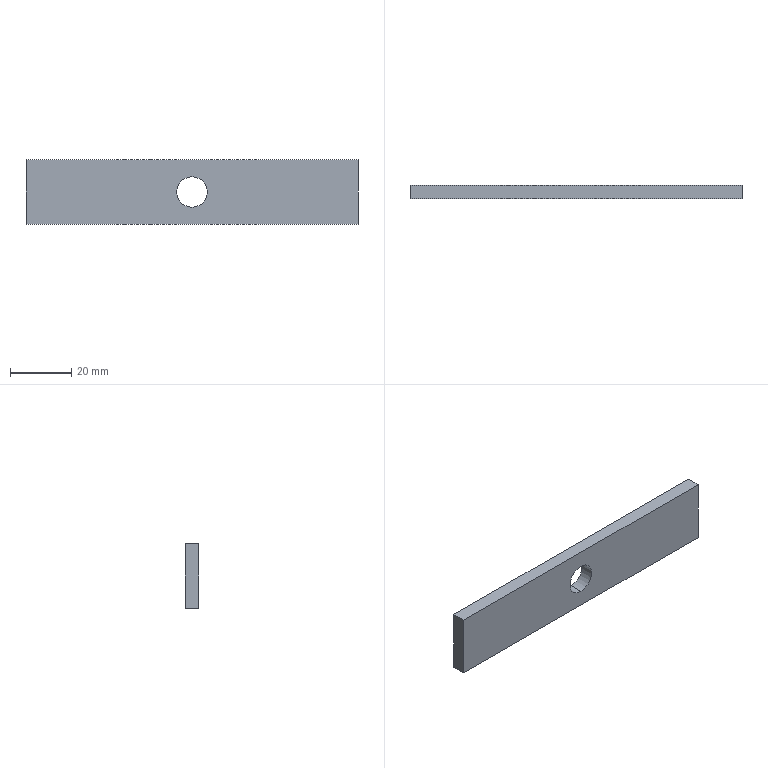Part | SolidWorks | features Extrusion 1 | 1 solid | 8 faces | box 108.732 x 4.5 x 21.168 mm | volume 10004 mm3 | plane 6 | cylinder 2 | commonest cylinder face diameters 10 x2
STEP:
#1=CARTESIAN_POINT('',(54.366,4.5,-15.584));
#2=VERTEX_POINT('',#1);
#3=CARTESIAN_POINT('',(54.366,4.5,-5.584));
#4=VERTEX_POINT('',#3);
#5=CARTESIAN_POINT('',(54.366,4.5,-10.584));
#6=DIRECTION('',(0.,1.,0.));
#7=DIRECTION('',(0.,0.,1.));
#8=AXIS2_PLACEMENT_3D('',#5,#6,#7);
#9=CIRCLE('',#8,5.);
#10=EDGE_CURVE('',#2,#4,#9,.T.);
#11=ORIENTED_EDGE('',*,*,#10,.T.);
#12=CARTESIAN_POINT('',(54.366,0.,-5.584));
#13=VERTEX_POINT('',#12);
#14=CARTESIAN_POINT('',(54.366,4.5,-5.584));
#15=DIRECTION('',(0.,-1.,0.));
#16=VECTOR('',#15,1000.);
#17=LINE('',#14,#16);
#18=EDGE_CURVE('',#4,#13,#17,.T.);
#19=ORIENTED_EDGE('',*,*,#18,.T.);
#20=CARTESIAN_POINT('',(54.366,0.,-15.584));
#21=VERTEX_POINT('',#20);
#22=CARTESIAN_POINT('',(54.366,0.,-10.584));
#23=DIRECTION('',(0.,1.,0.));
#24=DIRECTION('',(0.,0.,1.));
#25=AXIS2_PLACEMENT_3D('',#22,#23,#24);
#26=CIRCLE('',#25,5.);
#27=EDGE_CURVE('',#21,#13,#26,.T.);
#28=ORIENTED_EDGE('',*,*,#27,.F.);
#29=CARTESIAN_POINT('',(54.366,4.5,-15.584));
#30=DIRECTION('',(0.,-1.,0.));
#31=VECTOR('',#30,1000.);
#32=LINE('',#29,#31);
#33=EDGE_CURVE('',#2,#21,#32,.T.);
#34=ORIENTED_EDGE('',*,*,#33,.F.);
#35=EDGE_LOOP('',(#11,#19,#28,#34));
#36=FACE_OUTER_BOUND('',#35,.T.);
#37=CARTESIAN_POINT('',(54.366,4.5,-10.584));
#38=DIRECTION('',(0.,-1.,0.));
#39=DIRECTION('',(0.,0.,-1.));
#40=AXIS2_PLACEMENT_3D('',#37,#38,#39);
#41=CYLINDRICAL_SURFACE('',#40,5.);
#42=ADVANCED_FACE('',(#36),#41,.F.);
#43=CARTESIAN_POINT('',(0.,4.5,-21.168));
#44=VERTEX_POINT('',#43);
#45=CARTESIAN_POINT('',(0.,4.5,0.));
#46=VERTEX_POINT('',#45);
#47=CARTESIAN_POINT('',(0.,4.5,0.));
#48=DIRECTION('',(0.,0.,1.));
#49=VECTOR('',#48,1000.);
#50=LINE('',#47,#49);
#51=EDGE_CURVE('',#44,#46,#50,.T.);
#52=ORIENTED_EDGE('',*,*,#51,.T.);
#53=CARTESIAN_POINT('',(108.732,4.5,0.));
#54=VERTEX_POINT('',#53);
#55=CARTESIAN_POINT('',(0.,4.5,0.));
#56=DIRECTION('',(1.,0.,0.));
#57=VECTOR('',#56,1000.);
#58=LINE('',#55,#57);
#59=EDGE_CURVE('',#46,#54,#58,.T.);
#60=ORIENTED_EDGE('',*,*,#59,.T.);
#61=CARTESIAN_POINT('',(108.732,4.5,-21.168));
#62=VERTEX_POINT('',#61);
#63=CARTESIAN_POINT('',(108.732,4.5,0.));
#64=DIRECTION('',(0.,0.,-1.));
#65=VECTOR('',#64,1000.);
#66=LINE('',#63,#65);
#67=EDGE_CURVE('',#54,#62,#66,.T.);
#68=ORIENTED_EDGE('',*,*,#67,.T.);
#69=CARTESIAN_POINT('',(0.,4.5,-21.168));
#70=DIRECTION('',(-1.,0.,0.));
#71=VECTOR('',#70,1000.);
#72=LINE('',#69,#71);
#73=EDGE_CURVE('',#62,#44,#72,.T.);
#74=ORIENTED_EDGE('',*,*,#73,.T.);
#75=EDGE_LOOP('',(#52,#60,#68,#74));
#76=FACE_OUTER_BOUND('',#75,.T.);
#77=ORIENTED_EDGE('',*,*,#10,.F.);
#78=CARTESIAN_POINT('',(54.366,4.5,-10.584));
#79=DIRECTION('',(0.,1.,0.));
#80=DIRECTION('',(0.,0.,1.));
#81=AXIS2_PLACEMENT_3D('',#78,#79,#80);
#82=CIRCLE('',#81,5.);
#83=EDGE_CURVE('',#4,#2,#82,.T.);
#84=ORIENTED_EDGE('',*,*,#83,.F.);
#85=EDGE_LOOP('',(#77,#84));
#86=FACE_BOUND('',#85,.T.);
#87=CARTESIAN_POINT('',(0.,4.5,0.));
#88=DIRECTION('',(0.,-1.,0.));
#89=DIRECTION('',(0.,0.,-1.));
#90=AXIS2_PLACEMENT_3D('',#87,#88,#89);
#91=PLANE('',#90);
#92=ADVANCED_FACE('',(#76,#86),#91,.F.);
#93=CARTESIAN_POINT('',(0.,0.,-21.168));
#94=VERTEX_POINT('',#93);
#95=CARTESIAN_POINT('',(0.,0.,0.));
#96=VERTEX_POINT('',#95);
#97=CARTESIAN_POINT('',(0.,0.,0.));
#98=DIRECTION('',(0.,0.,1.));
#99=VECTOR('',#98,1000.);
#100=LINE('',#97,#99);
#101=EDGE_CURVE('',#94,#96,#100,.T.);
#102=ORIENTED_EDGE('',*,*,#101,.F.);
#103=CARTESIAN_POINT('',(108.732,0.,-21.168));
#104=VERTEX_POINT('',#103);
#105=CARTESIAN_POINT('',(0.,0.,-21.168));
#106=DIRECTION('',(-1.,0.,0.));
#107=VECTOR('',#106,1000.);
#108=LINE('',#105,#107);
#109=EDGE_CURVE('',#104,#94,#108,.T.);
#110=ORIENTED_EDGE('',*,*,#109,.F.);
#111=CARTESIAN_POINT('',(108.732,0.,0.));
#112=VERTEX_POINT('',#111);
#113=CARTESIAN_POINT('',(108.732,0.,0.));
#114=DIRECTION('',(0.,0.,-1.));
#115=VECTOR('',#114,1000.);
#116=LINE('',#113,#115);
#117=EDGE_CURVE('',#112,#104,#116,.T.);
#118=ORIENTED_EDGE('',*,*,#117,.F.);
#119=CARTESIAN_POINT('',(0.,0.,0.));
#120=DIRECTION('',(1.,0.,0.));
#121=VECTOR('',#120,1000.);
#122=LINE('',#119,#121);
#123=EDGE_CURVE('',#96,#112,#122,.T.);
#124=ORIENTED_EDGE('',*,*,#123,.F.);
#125=EDGE_LOOP('',(#102,#110,#118,#124));
#126=FACE_OUTER_BOUND('',#125,.T.);
#127=ORIENTED_EDGE('',*,*,#27,.T.);
#128=CARTESIAN_POINT('',(54.366,0.,-10.584));
#129=DIRECTION('',(0.,1.,0.));
#130=DIRECTION('',(0.,0.,1.));
#131=AXIS2_PLACEMENT_3D('',#128,#129,#130);
#132=CIRCLE('',#131,5.);
#133=EDGE_CURVE('',#13,#21,#132,.T.);
#134=ORIENTED_EDGE('',*,*,#133,.T.);
#135=EDGE_LOOP('',(#127,#134));
#136=FACE_BOUND('',#135,.T.);
#137=CARTESIAN_POINT('',(0.,0.,0.));
#138=DIRECTION('',(0.,-1.,0.));
#139=DIRECTION('',(0.,0.,-1.));
#140=AXIS2_PLACEMENT_3D('',#137,#138,#139);
#141=PLANE('',#140);
#142=ADVANCED_FACE('',(#126,#136),#141,.T.);
#143=ORIENTED_EDGE('',*,*,#101,.T.);
#144=CARTESIAN_POINT('',(0.,4.5,0.));
#145=DIRECTION('',(0.,-1.,0.));
#146=VECTOR('',#145,1000.);
#147=LINE('',#144,#146);
#148=EDGE_CURVE('',#46,#96,#147,.T.);
#149=ORIENTED_EDGE('',*,*,#148,.F.);
#150=ORIENTED_EDGE('',*,*,#51,.F.);
#151=CARTESIAN_POINT('',(0.,4.5,-21.168));
#152=DIRECTION('',(0.,-1.,0.));
#153=VECTOR('',#152,1000.);
#154=LINE('',#151,#153);
#155=EDGE_CURVE('',#44,#94,#154,.T.);
#156=ORIENTED_EDGE('',*,*,#155,.T.);
#157=EDGE_LOOP('',(#143,#149,#150,#156));
#158=FACE_OUTER_BOUND('',#157,.T.);
#159=CARTESIAN_POINT('',(0.,4.5,0.));
#160=DIRECTION('',(1.,0.,0.));
#161=DIRECTION('',(0.,0.,-1.));
#162=AXIS2_PLACEMENT_3D('',#159,#160,#161);
#163=PLANE('',#162);
#164=ADVANCED_FACE('',(#158),#163,.F.);
#165=ORIENTED_EDGE('',*,*,#123,.T.);
#166=CARTESIAN_POINT('',(108.732,4.5,0.));
#167=DIRECTION('',(0.,-1.,0.));
#168=VECTOR('',#167,1000.);
#169=LINE('',#166,#168);
#170=EDGE_CURVE('',#54,#112,#169,.T.);
#171=ORIENTED_EDGE('',*,*,#170,.F.);
#172=ORIENTED_EDGE('',*,*,#59,.F.);
#173=ORIENTED_EDGE('',*,*,#148,.T.);
#174=EDGE_LOOP('',(#165,#171,#172,#173));
#175=FACE_OUTER_BOUND('',#174,.T.);
#176=CARTESIAN_POINT('',(0.,4.5,0.));
#177=DIRECTION('',(0.,0.,-1.));
#178=DIRECTION('',(-1.,0.,0.));
#179=AXIS2_PLACEMENT_3D('',#176,#177,#178);
#180=PLANE('',#179);
#181=ADVANCED_FACE('',(#175),#180,.F.);
#182=ORIENTED_EDGE('',*,*,#117,.T.);
#183=CARTESIAN_POINT('',(108.732,4.5,-21.168));
#184=DIRECTION('',(0.,-1.,0.));
#185=VECTOR('',#184,1000.);
#186=LINE('',#183,#185);
#187=EDGE_CURVE('',#62,#104,#186,.T.);
#188=ORIENTED_EDGE('',*,*,#187,.F.);
#189=ORIENTED_EDGE('',*,*,#67,.F.);
#190=ORIENTED_EDGE('',*,*,#170,.T.);
#191=EDGE_LOOP('',(#182,#188,#189,#190));
#192=FACE_OUTER_BOUND('',#191,.T.);
#193=CARTESIAN_POINT('',(108.732,4.5,0.));
#194=DIRECTION('',(-1.,0.,0.));
#195=DIRECTION('',(0.,0.,1.));
#196=AXIS2_PLACEMENT_3D('',#193,#194,#195);
#197=PLANE('',#196);
#198=ADVANCED_FACE('',(#192),#197,.F.);
#199=ORIENTED_EDGE('',*,*,#109,.T.);
#200=ORIENTED_EDGE('',*,*,#155,.F.);
#201=ORIENTED_EDGE('',*,*,#73,.F.);
#202=ORIENTED_EDGE('',*,*,#187,.T.);
#203=EDGE_LOOP('',(#199,#200,#201,#202));
#204=FACE_OUTER_BOUND('',#203,.T.);
#205=CARTESIAN_POINT('',(0.,4.5,-21.168));
#206=DIRECTION('',(0.,0.,1.));
#207=DIRECTION('',(1.,0.,0.));
#208=AXIS2_PLACEMENT_3D('',#205,#206,#207);
#209=PLANE('',#208);
#210=ADVANCED_FACE('',(#204),#209,.F.);
#211=ORIENTED_EDGE('',*,*,#18,.F.);
#212=ORIENTED_EDGE('',*,*,#83,.T.);
#213=ORIENTED_EDGE('',*,*,#33,.T.);
#214=ORIENTED_EDGE('',*,*,#133,.F.);
#215=EDGE_LOOP('',(#211,#212,#213,#214));
#216=FACE_OUTER_BOUND('',#215,.T.);
#217=CARTESIAN_POINT('',(54.366,4.5,-10.584));
#218=DIRECTION('',(0.,-1.,0.));
#219=DIRECTION('',(0.,0.,-1.));
#220=AXIS2_PLACEMENT_3D('',#217,#218,#219);
#221=CYLINDRICAL_SURFACE('',#220,5.);
#222=ADVANCED_FACE('',(#216),#221,.F.);
#223=CLOSED_SHELL('',(#42,#92,#142,#164,#181,#198,#210,#222));
#224=MANIFOLD_SOLID_BREP('',#223);
#225=CARTESIAN_POINT('',(0.,0.,0.));
#226=DIRECTION('',(0.,0.,1.));
#227=DIRECTION('',(1.,0.,0.));
#228=AXIS2_PLACEMENT_3D('',#225,#226,#227);
#229=(LENGTH_UNIT()NAMED_UNIT(*)SI_UNIT(.MILLI.,.METRE.));
#230=UNCERTAINTY_MEASURE_WITH_UNIT(LENGTH_MEASURE(0.00001),#229,'','');
#231=(NAMED_UNIT(*)PLANE_ANGLE_UNIT()SI_UNIT($,.RADIAN.));
#232=(NAMED_UNIT(*)SI_UNIT($,.STERADIAN.)SOLID_ANGLE_UNIT());
#233=(GEOMETRIC_REPRESENTATION_CONTEXT(3)GLOBAL_UNCERTAINTY_ASSIGNED_CONTEXT((#230))GLOBAL_UNIT_ASSIGNED_CONTEXT((#229,#231,#232))REPRESENTATION_CONTEXT('',''));
#234=ADVANCED_BREP_SHAPE_REPRESENTATION('',(#224,#228),#233);